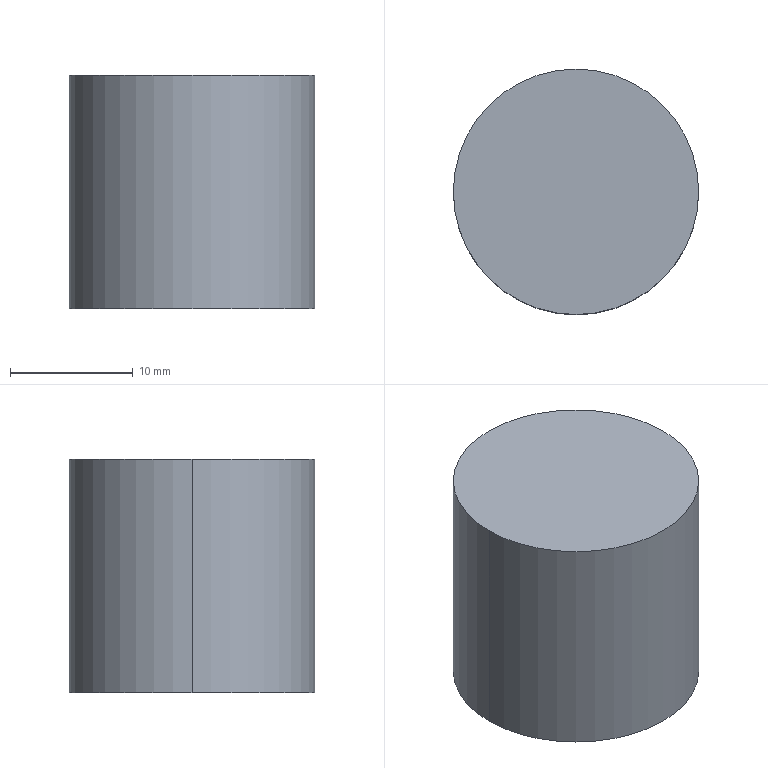Part | 1 solid | 4 faces | box 20 x 20 x 19 mm | volume 5969 mm3 | cylinder 2 | plane 2 | commonest cylinder face diameters 20 x2
STEP:
#1=CARTESIAN_POINT('',(10.,0.,19.));
#2=VERTEX_POINT('',#1);
#3=CARTESIAN_POINT('',(-10.,0.,19.));
#4=VERTEX_POINT('',#3);
#5=CARTESIAN_POINT('',(0.,0.,19.));
#6=DIRECTION('',(0.,0.,1.));
#7=DIRECTION('',(1.,0.,0.));
#8=AXIS2_PLACEMENT_3D('',#5,#6,#7);
#9=CIRCLE('',#8,10.);
#10=EDGE_CURVE('',#2,#4,#9,.T.);
#11=ORIENTED_EDGE('',*,*,#10,.F.);
#12=CARTESIAN_POINT('',(10.,0.,0.));
#13=VERTEX_POINT('',#12);
#14=CARTESIAN_POINT('',(10.,0.,19.));
#15=DIRECTION('',(0.,0.,-1.));
#16=VECTOR('',#15,1000.);
#17=LINE('',#14,#16);
#18=EDGE_CURVE('',#2,#13,#17,.T.);
#19=ORIENTED_EDGE('',*,*,#18,.T.);
#20=CARTESIAN_POINT('',(-10.,0.,0.));
#21=VERTEX_POINT('',#20);
#22=CARTESIAN_POINT('',(0.,0.,0.));
#23=DIRECTION('',(0.,0.,1.));
#24=DIRECTION('',(1.,0.,0.));
#25=AXIS2_PLACEMENT_3D('',#22,#23,#24);
#26=CIRCLE('',#25,10.);
#27=EDGE_CURVE('',#13,#21,#26,.T.);
#28=ORIENTED_EDGE('',*,*,#27,.T.);
#29=CARTESIAN_POINT('',(-10.,0.,19.));
#30=DIRECTION('',(0.,0.,-1.));
#31=VECTOR('',#30,1000.);
#32=LINE('',#29,#31);
#33=EDGE_CURVE('',#4,#21,#32,.T.);
#34=ORIENTED_EDGE('',*,*,#33,.F.);
#35=EDGE_LOOP('',(#11,#19,#28,#34));
#36=FACE_OUTER_BOUND('',#35,.T.);
#37=CARTESIAN_POINT('',(0.,0.,19.));
#38=DIRECTION('',(0.,0.,-1.));
#39=DIRECTION('',(-1.,0.,0.));
#40=AXIS2_PLACEMENT_3D('',#37,#38,#39);
#41=CYLINDRICAL_SURFACE('',#40,10.);
#42=ADVANCED_FACE('',(#36),#41,.T.);
#43=ORIENTED_EDGE('',*,*,#18,.F.);
#44=CARTESIAN_POINT('',(0.,0.,19.));
#45=DIRECTION('',(0.,0.,1.));
#46=DIRECTION('',(1.,0.,0.));
#47=AXIS2_PLACEMENT_3D('',#44,#45,#46);
#48=CIRCLE('',#47,10.);
#49=EDGE_CURVE('',#4,#2,#48,.T.);
#50=ORIENTED_EDGE('',*,*,#49,.F.);
#51=ORIENTED_EDGE('',*,*,#33,.T.);
#52=CARTESIAN_POINT('',(0.,0.,0.));
#53=DIRECTION('',(0.,0.,1.));
#54=DIRECTION('',(1.,0.,0.));
#55=AXIS2_PLACEMENT_3D('',#52,#53,#54);
#56=CIRCLE('',#55,10.);
#57=EDGE_CURVE('',#21,#13,#56,.T.);
#58=ORIENTED_EDGE('',*,*,#57,.T.);
#59=EDGE_LOOP('',(#43,#50,#51,#58));
#60=FACE_OUTER_BOUND('',#59,.T.);
#61=CARTESIAN_POINT('',(0.,0.,19.));
#62=DIRECTION('',(0.,0.,-1.));
#63=DIRECTION('',(-1.,0.,0.));
#64=AXIS2_PLACEMENT_3D('',#61,#62,#63);
#65=CYLINDRICAL_SURFACE('',#64,10.);
#66=ADVANCED_FACE('',(#60),#65,.T.);
#67=ORIENTED_EDGE('',*,*,#49,.T.);
#68=ORIENTED_EDGE('',*,*,#10,.T.);
#69=EDGE_LOOP('',(#67,#68));
#70=FACE_OUTER_BOUND('',#69,.T.);
#71=CARTESIAN_POINT('',(0.,0.,19.));
#72=DIRECTION('',(0.,0.,1.));
#73=DIRECTION('',(1.,0.,0.));
#74=AXIS2_PLACEMENT_3D('',#71,#72,#73);
#75=PLANE('',#74);
#76=ADVANCED_FACE('',(#70),#75,.T.);
#77=ORIENTED_EDGE('',*,*,#57,.F.);
#78=ORIENTED_EDGE('',*,*,#27,.F.);
#79=EDGE_LOOP('',(#77,#78));
#80=FACE_OUTER_BOUND('',#79,.T.);
#81=CARTESIAN_POINT('',(0.,0.,0.));
#82=DIRECTION('',(0.,0.,1.));
#83=DIRECTION('',(1.,0.,0.));
#84=AXIS2_PLACEMENT_3D('',#81,#82,#83);
#85=PLANE('',#84);
#86=ADVANCED_FACE('',(#80),#85,.F.);
#87=CLOSED_SHELL('',(#42,#66,#76,#86));
#88=MANIFOLD_SOLID_BREP('',#87);
#89=CARTESIAN_POINT('',(0.,0.,0.));
#90=DIRECTION('',(0.,0.,1.));
#91=DIRECTION('',(1.,0.,0.));
#92=AXIS2_PLACEMENT_3D('',#89,#90,#91);
#93=(LENGTH_UNIT()NAMED_UNIT(*)SI_UNIT(.MILLI.,.METRE.));
#94=UNCERTAINTY_MEASURE_WITH_UNIT(LENGTH_MEASURE(0.00001),#93,'','');
#95=(NAMED_UNIT(*)PLANE_ANGLE_UNIT()SI_UNIT($,.RADIAN.));
#96=(NAMED_UNIT(*)SI_UNIT($,.STERADIAN.)SOLID_ANGLE_UNIT());
#97=(GEOMETRIC_REPRESENTATION_CONTEXT(3)GLOBAL_UNCERTAINTY_ASSIGNED_CONTEXT((#94))GLOBAL_UNIT_ASSIGNED_CONTEXT((#93,#95,#96))REPRESENTATION_CONTEXT('',''));
#98=ADVANCED_BREP_SHAPE_REPRESENTATION('',(#88,#92),#97);